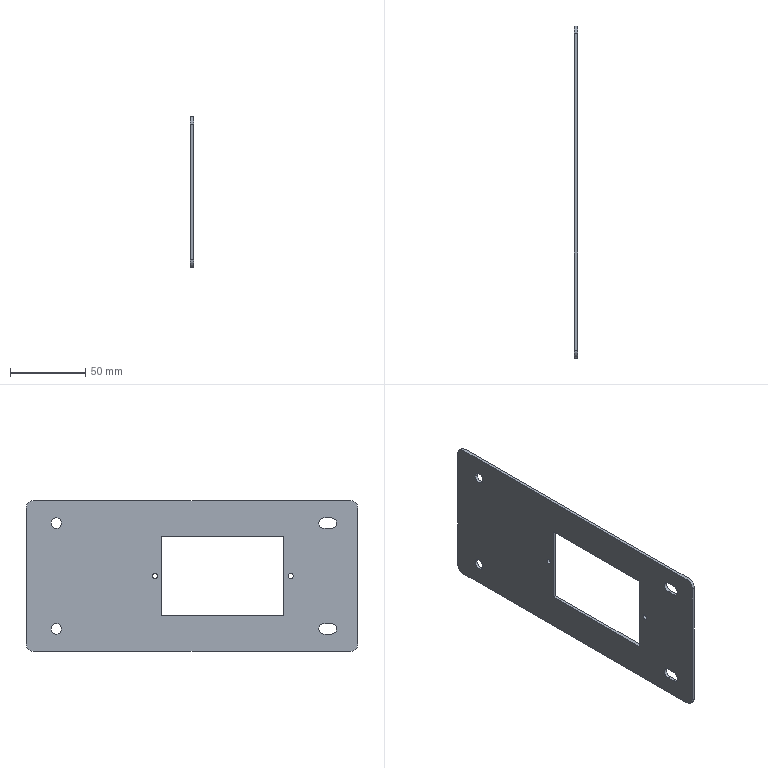Part | SolidWorks | features ExtruThin 1, Fillet 1, ICE 1 | 1 solid | 32 faces | box 2 x 220 x 100 mm | volume 34889 mm3 | cylinder 18 | plane 14 | commonest cylinder face diameters 7 x10 3.3 x4 10 x4
STEP:
#1=CARTESIAN_POINT('',(2.,14.,-85.));
#2=VERTEX_POINT('',#1);
#3=CARTESIAN_POINT('',(2.,17.5,-81.5));
#4=VERTEX_POINT('',#3);
#5=CARTESIAN_POINT('',(2.,17.5,-85.));
#6=DIRECTION('',(-1.,0.,0.));
#7=DIRECTION('',(0.,-1.,0.));
#8=AXIS2_PLACEMENT_3D('',#5,#6,#7);
#9=CIRCLE('',#8,3.5);
#10=EDGE_CURVE('',#2,#4,#9,.T.);
#11=ORIENTED_EDGE('',*,*,#10,.F.);
#12=CARTESIAN_POINT('',(0.,14.,-85.));
#13=VERTEX_POINT('',#12);
#14=CARTESIAN_POINT('',(10.,14.,-85.));
#15=DIRECTION('',(-1.,0.,0.));
#16=VECTOR('',#15,1000.);
#17=LINE('',#14,#16);
#18=EDGE_CURVE('',#2,#13,#17,.T.);
#19=ORIENTED_EDGE('',*,*,#18,.T.);
#20=CARTESIAN_POINT('',(0.,17.5,-81.5));
#21=VERTEX_POINT('',#20);
#22=CARTESIAN_POINT('',(0.,17.5,-85.));
#23=DIRECTION('',(-1.,0.,0.));
#24=DIRECTION('',(0.,-1.,0.));
#25=AXIS2_PLACEMENT_3D('',#22,#23,#24);
#26=CIRCLE('',#25,3.5);
#27=EDGE_CURVE('',#13,#21,#26,.T.);
#28=ORIENTED_EDGE('',*,*,#27,.T.);
#29=CARTESIAN_POINT('',(10.,17.5,-81.5));
#30=DIRECTION('',(-1.,0.,0.));
#31=VECTOR('',#30,1000.);
#32=LINE('',#29,#31);
#33=EDGE_CURVE('',#4,#21,#32,.T.);
#34=ORIENTED_EDGE('',*,*,#33,.F.);
#35=EDGE_LOOP('',(#11,#19,#28,#34));
#36=FACE_OUTER_BOUND('',#35,.T.);
#37=CARTESIAN_POINT('',(10.,17.5,-85.));
#38=DIRECTION('',(-1.,0.,0.));
#39=DIRECTION('',(0.,-1.,0.));
#40=AXIS2_PLACEMENT_3D('',#37,#38,#39);
#41=CYLINDRICAL_SURFACE('',#40,3.5);
#42=ADVANCED_FACE('',(#36),#41,.F.);
#43=CARTESIAN_POINT('',(2.,14.,-15.));
#44=VERTEX_POINT('',#43);
#45=CARTESIAN_POINT('',(2.,17.5,-11.5));
#46=VERTEX_POINT('',#45);
#47=CARTESIAN_POINT('',(2.,17.5,-15.));
#48=DIRECTION('',(-1.,0.,0.));
#49=DIRECTION('',(0.,-1.,0.));
#50=AXIS2_PLACEMENT_3D('',#47,#48,#49);
#51=CIRCLE('',#50,3.5);
#52=EDGE_CURVE('',#44,#46,#51,.T.);
#53=ORIENTED_EDGE('',*,*,#52,.F.);
#54=CARTESIAN_POINT('',(0.,14.,-15.));
#55=VERTEX_POINT('',#54);
#56=CARTESIAN_POINT('',(10.,14.,-15.));
#57=DIRECTION('',(-1.,0.,0.));
#58=VECTOR('',#57,1000.);
#59=LINE('',#56,#58);
#60=EDGE_CURVE('',#44,#55,#59,.T.);
#61=ORIENTED_EDGE('',*,*,#60,.T.);
#62=CARTESIAN_POINT('',(0.,17.5,-11.5));
#63=VERTEX_POINT('',#62);
#64=CARTESIAN_POINT('',(0.,17.5,-15.));
#65=DIRECTION('',(-1.,0.,0.));
#66=DIRECTION('',(0.,-1.,0.));
#67=AXIS2_PLACEMENT_3D('',#64,#65,#66);
#68=CIRCLE('',#67,3.5);
#69=EDGE_CURVE('',#55,#63,#68,.T.);
#70=ORIENTED_EDGE('',*,*,#69,.T.);
#71=CARTESIAN_POINT('',(10.,17.5,-11.5));
#72=DIRECTION('',(-1.,0.,0.));
#73=VECTOR('',#72,1000.);
#74=LINE('',#71,#73);
#75=EDGE_CURVE('',#46,#63,#74,.T.);
#76=ORIENTED_EDGE('',*,*,#75,.F.);
#77=EDGE_LOOP('',(#53,#61,#70,#76));
#78=FACE_OUTER_BOUND('',#77,.T.);
#79=CARTESIAN_POINT('',(10.,17.5,-15.));
#80=DIRECTION('',(-1.,0.,0.));
#81=DIRECTION('',(0.,-1.,0.));
#82=AXIS2_PLACEMENT_3D('',#79,#80,#81);
#83=CYLINDRICAL_SURFACE('',#82,3.5);
#84=ADVANCED_FACE('',(#78),#83,.F.);
#85=CARTESIAN_POINT('',(2.,203.5,-85.));
#86=VERTEX_POINT('',#85);
#87=CARTESIAN_POINT('',(2.,196.5,-85.));
#88=VERTEX_POINT('',#87);
#89=CARTESIAN_POINT('',(2.,200.,-85.));
#90=DIRECTION('',(-1.,0.,0.));
#91=DIRECTION('',(0.,-1.,0.));
#92=AXIS2_PLACEMENT_3D('',#89,#90,#91);
#93=CIRCLE('',#92,3.5);
#94=EDGE_CURVE('',#86,#88,#93,.T.);
#95=ORIENTED_EDGE('',*,*,#94,.F.);
#96=CARTESIAN_POINT('',(0.,203.5,-85.));
#97=VERTEX_POINT('',#96);
#98=CARTESIAN_POINT('',(10.,203.5,-85.));
#99=DIRECTION('',(-1.,0.,0.));
#100=VECTOR('',#99,1000.);
#101=LINE('',#98,#100);
#102=EDGE_CURVE('',#86,#97,#101,.T.);
#103=ORIENTED_EDGE('',*,*,#102,.T.);
#104=CARTESIAN_POINT('',(0.,196.5,-85.));
#105=VERTEX_POINT('',#104);
#106=CARTESIAN_POINT('',(0.,200.,-85.));
#107=DIRECTION('',(-1.,0.,0.));
#108=DIRECTION('',(0.,-1.,0.));
#109=AXIS2_PLACEMENT_3D('',#106,#107,#108);
#110=CIRCLE('',#109,3.5);
#111=EDGE_CURVE('',#97,#105,#110,.T.);
#112=ORIENTED_EDGE('',*,*,#111,.T.);
#113=CARTESIAN_POINT('',(10.,196.5,-85.));
#114=DIRECTION('',(-1.,0.,0.));
#115=VECTOR('',#114,1000.);
#116=LINE('',#113,#115);
#117=EDGE_CURVE('',#88,#105,#116,.T.);
#118=ORIENTED_EDGE('',*,*,#117,.F.);
#119=EDGE_LOOP('',(#95,#103,#112,#118));
#120=FACE_OUTER_BOUND('',#119,.T.);
#121=CARTESIAN_POINT('',(10.,200.,-85.));
#122=DIRECTION('',(-1.,0.,0.));
#123=DIRECTION('',(0.,-1.,0.));
#124=AXIS2_PLACEMENT_3D('',#121,#122,#123);
#125=CYLINDRICAL_SURFACE('',#124,3.5);
#126=ADVANCED_FACE('',(#120),#125,.F.);
#127=CARTESIAN_POINT('',(2.,203.5,-15.));
#128=VERTEX_POINT('',#127);
#129=CARTESIAN_POINT('',(2.,196.5,-15.));
#130=VERTEX_POINT('',#129);
#131=CARTESIAN_POINT('',(2.,200.,-15.));
#132=DIRECTION('',(-1.,0.,0.));
#133=DIRECTION('',(0.,-1.,0.));
#134=AXIS2_PLACEMENT_3D('',#131,#132,#133);
#135=CIRCLE('',#134,3.5);
#136=EDGE_CURVE('',#128,#130,#135,.T.);
#137=ORIENTED_EDGE('',*,*,#136,.F.);
#138=CARTESIAN_POINT('',(0.,203.5,-15.));
#139=VERTEX_POINT('',#138);
#140=CARTESIAN_POINT('',(10.,203.5,-15.));
#141=DIRECTION('',(-1.,0.,0.));
#142=VECTOR('',#141,1000.);
#143=LINE('',#140,#142);
#144=EDGE_CURVE('',#128,#139,#143,.T.);
#145=ORIENTED_EDGE('',*,*,#144,.T.);
#146=CARTESIAN_POINT('',(0.,196.5,-15.));
#147=VERTEX_POINT('',#146);
#148=CARTESIAN_POINT('',(0.,200.,-15.));
#149=DIRECTION('',(-1.,0.,0.));
#150=DIRECTION('',(0.,-1.,0.));
#151=AXIS2_PLACEMENT_3D('',#148,#149,#150);
#152=CIRCLE('',#151,3.5);
#153=EDGE_CURVE('',#139,#147,#152,.T.);
#154=ORIENTED_EDGE('',*,*,#153,.T.);
#155=CARTESIAN_POINT('',(10.,196.5,-15.));
#156=DIRECTION('',(-1.,0.,0.));
#157=VECTOR('',#156,1000.);
#158=LINE('',#155,#157);
#159=EDGE_CURVE('',#130,#147,#158,.T.);
#160=ORIENTED_EDGE('',*,*,#159,.F.);
#161=EDGE_LOOP('',(#137,#145,#154,#160));
#162=FACE_OUTER_BOUND('',#161,.T.);
#163=CARTESIAN_POINT('',(10.,200.,-15.));
#164=DIRECTION('',(-1.,0.,0.));
#165=DIRECTION('',(0.,-1.,0.));
#166=AXIS2_PLACEMENT_3D('',#163,#164,#165);
#167=CYLINDRICAL_SURFACE('',#166,3.5);
#168=ADVANCED_FACE('',(#162),#167,.F.);
#169=CARTESIAN_POINT('',(2.,136.15,-50.));
#170=VERTEX_POINT('',#169);
#171=CARTESIAN_POINT('',(2.,132.85,-50.));
#172=VERTEX_POINT('',#171);
#173=CARTESIAN_POINT('',(2.,134.5,-50.));
#174=DIRECTION('',(-1.,0.,0.));
#175=DIRECTION('',(0.,-1.,0.));
#176=AXIS2_PLACEMENT_3D('',#173,#174,#175);
#177=CIRCLE('',#176,1.65);
#178=EDGE_CURVE('',#170,#172,#177,.T.);
#179=ORIENTED_EDGE('',*,*,#178,.F.);
#180=CARTESIAN_POINT('',(0.,136.15,-50.));
#181=VERTEX_POINT('',#180);
#182=CARTESIAN_POINT('',(10.,136.15,-50.));
#183=DIRECTION('',(-1.,0.,0.));
#184=VECTOR('',#183,1000.);
#185=LINE('',#182,#184);
#186=EDGE_CURVE('',#170,#181,#185,.T.);
#187=ORIENTED_EDGE('',*,*,#186,.T.);
#188=CARTESIAN_POINT('',(0.,132.85,-50.));
#189=VERTEX_POINT('',#188);
#190=CARTESIAN_POINT('',(0.,134.5,-50.));
#191=DIRECTION('',(-1.,0.,0.));
#192=DIRECTION('',(0.,-1.,0.));
#193=AXIS2_PLACEMENT_3D('',#190,#191,#192);
#194=CIRCLE('',#193,1.65);
#195=EDGE_CURVE('',#181,#189,#194,.T.);
#196=ORIENTED_EDGE('',*,*,#195,.T.);
#197=CARTESIAN_POINT('',(10.,132.85,-50.));
#198=DIRECTION('',(-1.,0.,0.));
#199=VECTOR('',#198,1000.);
#200=LINE('',#197,#199);
#201=EDGE_CURVE('',#172,#189,#200,.T.);
#202=ORIENTED_EDGE('',*,*,#201,.F.);
#203=EDGE_LOOP('',(#179,#187,#196,#202));
#204=FACE_OUTER_BOUND('',#203,.T.);
#205=CARTESIAN_POINT('',(10.,134.5,-50.));
#206=DIRECTION('',(-1.,0.,0.));
#207=DIRECTION('',(0.,-1.,0.));
#208=AXIS2_PLACEMENT_3D('',#205,#206,#207);
#209=CYLINDRICAL_SURFACE('',#208,1.65);
#210=ADVANCED_FACE('',(#204),#209,.F.);
#211=CARTESIAN_POINT('',(2.,46.15,-50.));
#212=VERTEX_POINT('',#211);
#213=CARTESIAN_POINT('',(2.,42.85,-50.));
#214=VERTEX_POINT('',#213);
#215=CARTESIAN_POINT('',(2.,44.5,-50.));
#216=DIRECTION('',(-1.,0.,0.));
#217=DIRECTION('',(0.,-1.,0.));
#218=AXIS2_PLACEMENT_3D('',#215,#216,#217);
#219=CIRCLE('',#218,1.65);
#220=EDGE_CURVE('',#212,#214,#219,.T.);
#221=ORIENTED_EDGE('',*,*,#220,.F.);
#222=CARTESIAN_POINT('',(0.,46.15,-50.));
#223=VERTEX_POINT('',#222);
#224=CARTESIAN_POINT('',(10.,46.15,-50.));
#225=DIRECTION('',(-1.,0.,0.));
#226=VECTOR('',#225,1000.);
#227=LINE('',#224,#226);
#228=EDGE_CURVE('',#212,#223,#227,.T.);
#229=ORIENTED_EDGE('',*,*,#228,.T.);
#230=CARTESIAN_POINT('',(0.,42.85,-50.));
#231=VERTEX_POINT('',#230);
#232=CARTESIAN_POINT('',(0.,44.5,-50.));
#233=DIRECTION('',(-1.,0.,0.));
#234=DIRECTION('',(0.,-1.,0.));
#235=AXIS2_PLACEMENT_3D('',#232,#233,#234);
#236=CIRCLE('',#235,1.65);
#237=EDGE_CURVE('',#223,#231,#236,.T.);
#238=ORIENTED_EDGE('',*,*,#237,.T.);
#239=CARTESIAN_POINT('',(10.,42.85,-50.));
#240=DIRECTION('',(-1.,0.,0.));
#241=VECTOR('',#240,1000.);
#242=LINE('',#239,#241);
#243=EDGE_CURVE('',#214,#231,#242,.T.);
#244=ORIENTED_EDGE('',*,*,#243,.F.);
#245=EDGE_LOOP('',(#221,#229,#238,#244));
#246=FACE_OUTER_BOUND('',#245,.T.);
#247=CARTESIAN_POINT('',(10.,44.5,-50.));
#248=DIRECTION('',(-1.,0.,0.));
#249=DIRECTION('',(0.,-1.,0.));
#250=AXIS2_PLACEMENT_3D('',#247,#248,#249);
#251=CYLINDRICAL_SURFACE('',#250,1.65);
#252=ADVANCED_FACE('',(#246),#251,.F.);
#253=CARTESIAN_POINT('',(0.,22.5,-81.5));
#254=VERTEX_POINT('',#253);
#255=CARTESIAN_POINT('',(0.,22.5,-88.5));
#256=VERTEX_POINT('',#255);
#257=CARTESIAN_POINT('',(0.,22.5,-85.));
#258=DIRECTION('',(-1.,0.,0.));
#259=DIRECTION('',(0.,-1.,0.));
#260=AXIS2_PLACEMENT_3D('',#257,#258,#259);
#261=CIRCLE('',#260,3.5);
#262=EDGE_CURVE('',#254,#256,#261,.T.);
#263=ORIENTED_EDGE('',*,*,#262,.F.);
#264=CARTESIAN_POINT('',(0.,22.5,-81.5));
#265=DIRECTION('',(0.,1.,0.));
#266=VECTOR('',#265,1000.);
#267=LINE('',#264,#266);
#268=EDGE_CURVE('',#21,#254,#267,.T.);
#269=ORIENTED_EDGE('',*,*,#268,.F.);
#270=ORIENTED_EDGE('',*,*,#27,.F.);
#271=CARTESIAN_POINT('',(0.,17.5,-88.5));
#272=VERTEX_POINT('',#271);
#273=CARTESIAN_POINT('',(0.,17.5,-85.));
#274=DIRECTION('',(-1.,0.,0.));
#275=DIRECTION('',(0.,-1.,0.));
#276=AXIS2_PLACEMENT_3D('',#273,#274,#275);
#277=CIRCLE('',#276,3.5);
#278=EDGE_CURVE('',#272,#13,#277,.T.);
#279=ORIENTED_EDGE('',*,*,#278,.F.);
#280=CARTESIAN_POINT('',(0.,22.5,-88.5));
#281=DIRECTION('',(0.,-1.,0.));
#282=VECTOR('',#281,1000.);
#283=LINE('',#280,#282);
#284=EDGE_CURVE('',#256,#272,#283,.T.);
#285=ORIENTED_EDGE('',*,*,#284,.F.);
#286=EDGE_LOOP('',(#263,#269,#270,#279,#285));
#287=FACE_BOUND('',#286,.T.);
#288=CARTESIAN_POINT('',(0.,22.5,-11.5));
#289=VERTEX_POINT('',#288);
#290=CARTESIAN_POINT('',(0.,22.5,-18.5));
#291=VERTEX_POINT('',#290);
#292=CARTESIAN_POINT('',(0.,22.5,-15.));
#293=DIRECTION('',(-1.,0.,0.));
#294=DIRECTION('',(0.,-1.,0.));
#295=AXIS2_PLACEMENT_3D('',#292,#293,#294);
#296=CIRCLE('',#295,3.5);
#297=EDGE_CURVE('',#289,#291,#296,.T.);
#298=ORIENTED_EDGE('',*,*,#297,.F.);
#299=CARTESIAN_POINT('',(0.,22.5,-11.5));
#300=DIRECTION('',(0.,1.,0.));
#301=VECTOR('',#300,1000.);
#302=LINE('',#299,#301);
#303=EDGE_CURVE('',#63,#289,#302,.T.);
#304=ORIENTED_EDGE('',*,*,#303,.F.);
#305=ORIENTED_EDGE('',*,*,#69,.F.);
#306=CARTESIAN_POINT('',(0.,17.5,-18.5));
#307=VERTEX_POINT('',#306);
#308=CARTESIAN_POINT('',(0.,17.5,-15.));
#309=DIRECTION('',(-1.,0.,0.));
#310=DIRECTION('',(0.,-1.,0.));
#311=AXIS2_PLACEMENT_3D('',#308,#309,#310);
#312=CIRCLE('',#311,3.5);
#313=EDGE_CURVE('',#307,#55,#312,.T.);
#314=ORIENTED_EDGE('',*,*,#313,.F.);
#315=CARTESIAN_POINT('',(0.,22.5,-18.5));
#316=DIRECTION('',(0.,-1.,0.));
#317=VECTOR('',#316,1000.);
#318=LINE('',#315,#317);
#319=EDGE_CURVE('',#291,#307,#318,.T.);
#320=ORIENTED_EDGE('',*,*,#319,.F.);
#321=EDGE_LOOP('',(#298,#304,#305,#314,#320));
#322=FACE_BOUND('',#321,.T.);
#323=CARTESIAN_POINT('',(0.,200.,-85.));
#324=DIRECTION('',(-1.,0.,0.));
#325=DIRECTION('',(0.,-1.,0.));
#326=AXIS2_PLACEMENT_3D('',#323,#324,#325);
#327=CIRCLE('',#326,3.5);
#328=EDGE_CURVE('',#105,#97,#327,.T.);
#329=ORIENTED_EDGE('',*,*,#328,.F.);
#330=ORIENTED_EDGE('',*,*,#111,.F.);
#331=EDGE_LOOP('',(#329,#330));
#332=FACE_BOUND('',#331,.T.);
#333=CARTESIAN_POINT('',(0.,200.,-15.));
#334=DIRECTION('',(-1.,0.,0.));
#335=DIRECTION('',(0.,-1.,0.));
#336=AXIS2_PLACEMENT_3D('',#333,#334,#335);
#337=CIRCLE('',#336,3.5);
#338=EDGE_CURVE('',#147,#139,#337,.T.);
#339=ORIENTED_EDGE('',*,*,#338,.F.);
#340=ORIENTED_EDGE('',*,*,#153,.F.);
#341=EDGE_LOOP('',(#339,#340));
#342=FACE_BOUND('',#341,.T.);
#343=CARTESIAN_POINT('',(0.,134.5,-50.));
#344=DIRECTION('',(-1.,0.,0.));
#345=DIRECTION('',(0.,-1.,0.));
#346=AXIS2_PLACEMENT_3D('',#343,#344,#345);
#347=CIRCLE('',#346,1.65);
#348=EDGE_CURVE('',#189,#181,#347,.T.);
#349=ORIENTED_EDGE('',*,*,#348,.F.);
#350=ORIENTED_EDGE('',*,*,#195,.F.);
#351=EDGE_LOOP('',(#349,#350));
#352=FACE_BOUND('',#351,.T.);
#353=CARTESIAN_POINT('',(0.,44.5,-50.));
#354=DIRECTION('',(-1.,0.,0.));
#355=DIRECTION('',(0.,-1.,0.));
#356=AXIS2_PLACEMENT_3D('',#353,#354,#355);
#357=CIRCLE('',#356,1.65);
#358=EDGE_CURVE('',#231,#223,#357,.T.);
#359=ORIENTED_EDGE('',*,*,#358,.F.);
#360=ORIENTED_EDGE('',*,*,#237,.F.);
#361=EDGE_LOOP('',(#359,#360));
#362=FACE_BOUND('',#361,.T.);
#363=CARTESIAN_POINT('',(0.,130.,-76.5));
#364=VERTEX_POINT('',#363);
#365=CARTESIAN_POINT('',(0.,49.,-76.5));
#366=VERTEX_POINT('',#365);
#367=CARTESIAN_POINT('',(0.,130.,-76.5));
#368=DIRECTION('',(0.,-1.,0.));
#369=VECTOR('',#368,1000.);
#370=LINE('',#367,#369);
#371=EDGE_CURVE('',#364,#366,#370,.T.);
#372=ORIENTED_EDGE('',*,*,#371,.F.);
#373=CARTESIAN_POINT('',(0.,130.,-23.5));
#374=VERTEX_POINT('',#373);
#375=CARTESIAN_POINT('',(0.,130.,-23.5));
#376=DIRECTION('',(0.,0.,-1.));
#377=VECTOR('',#376,1000.);
#378=LINE('',#375,#377);
#379=EDGE_CURVE('',#374,#364,#378,.T.);
#380=ORIENTED_EDGE('',*,*,#379,.F.);
#381=CARTESIAN_POINT('',(0.,49.,-23.5));
#382=VERTEX_POINT('',#381);
#383=CARTESIAN_POINT('',(0.,130.,-23.5));
#384=DIRECTION('',(0.,1.,0.));
#385=VECTOR('',#384,1000.);
#386=LINE('',#383,#385);
#387=EDGE_CURVE('',#382,#374,#386,.T.);
#388=ORIENTED_EDGE('',*,*,#387,.F.);
#389=CARTESIAN_POINT('',(0.,49.,-23.5));
#390=DIRECTION('',(0.,0.,1.));
#391=VECTOR('',#390,1000.);
#392=LINE('',#389,#391);
#393=EDGE_CURVE('',#366,#382,#392,.T.);
#394=ORIENTED_EDGE('',*,*,#393,.F.);
#395=EDGE_LOOP('',(#372,#380,#388,#394));
#396=FACE_BOUND('',#395,.T.);
#397=CARTESIAN_POINT('',(0.,220.,-95.));
#398=VERTEX_POINT('',#397);
#399=CARTESIAN_POINT('',(0.,220.,-5.));
#400=VERTEX_POINT('',#399);
#401=CARTESIAN_POINT('',(0.,220.,-100.));
#402=DIRECTION('',(0.,0.,1.));
#403=VECTOR('',#402,1000.);
#404=LINE('',#401,#403);
#405=EDGE_CURVE('',#398,#400,#404,.T.);
#406=ORIENTED_EDGE('',*,*,#405,.F.);
#407=CARTESIAN_POINT('',(0.,215.,-100.));
#408=VERTEX_POINT('',#407);
#409=CARTESIAN_POINT('',(0.,215.,-95.));
#410=DIRECTION('',(-1.,0.,0.));
#411=DIRECTION('',(0.,-1.,0.));
#412=AXIS2_PLACEMENT_3D('',#409,#410,#411);
#413=CIRCLE('',#412,5.);
#414=EDGE_CURVE('',#398,#408,#413,.T.);
#415=ORIENTED_EDGE('',*,*,#414,.T.);
#416=CARTESIAN_POINT('',(0.,5.,-100.));
#417=VERTEX_POINT('',#416);
#418=CARTESIAN_POINT('',(0.,220.,-100.));
#419=DIRECTION('',(0.,-1.,0.));
#420=VECTOR('',#419,1000.);
#421=LINE('',#418,#420);
#422=EDGE_CURVE('',#408,#417,#421,.T.);
#423=ORIENTED_EDGE('',*,*,#422,.T.);
#424=CARTESIAN_POINT('',(0.,0.,-95.));
#425=VERTEX_POINT('',#424);
#426=CARTESIAN_POINT('',(0.,5.,-95.));
#427=DIRECTION('',(-1.,0.,0.));
#428=DIRECTION('',(0.,-1.,0.));
#429=AXIS2_PLACEMENT_3D('',#426,#427,#428);
#430=CIRCLE('',#429,5.);
#431=EDGE_CURVE('',#417,#425,#430,.T.);
#432=ORIENTED_EDGE('',*,*,#431,.T.);
#433=CARTESIAN_POINT('',(0.,0.,-5.));
#434=VERTEX_POINT('',#433);
#435=CARTESIAN_POINT('',(0.,0.,-100.));
#436=DIRECTION('',(0.,0.,1.));
#437=VECTOR('',#436,1000.);
#438=LINE('',#435,#437);
#439=EDGE_CURVE('',#425,#434,#438,.T.);
#440=ORIENTED_EDGE('',*,*,#439,.T.);
#441=CARTESIAN_POINT('',(0.,5.,0.));
#442=VERTEX_POINT('',#441);
#443=CARTESIAN_POINT('',(0.,5.,-5.));
#444=DIRECTION('',(-1.,0.,0.));
#445=DIRECTION('',(0.,-1.,0.));
#446=AXIS2_PLACEMENT_3D('',#443,#444,#445);
#447=CIRCLE('',#446,5.);
#448=EDGE_CURVE('',#434,#442,#447,.T.);
#449=ORIENTED_EDGE('',*,*,#448,.T.);
#450=CARTESIAN_POINT('',(0.,215.,0.));
#451=VERTEX_POINT('',#450);
#452=CARTESIAN_POINT('',(0.,220.,0.));
#453=DIRECTION('',(0.,-1.,0.));
#454=VECTOR('',#453,1000.);
#455=LINE('',#452,#454);
#456=EDGE_CURVE('',#451,#442,#455,.T.);
#457=ORIENTED_EDGE('',*,*,#456,.F.);
#458=CARTESIAN_POINT('',(0.,215.,-5.));
#459=DIRECTION('',(-1.,0.,0.));
#460=DIRECTION('',(0.,-1.,0.));
#461=AXIS2_PLACEMENT_3D('',#458,#459,#460);
#462=CIRCLE('',#461,5.);
#463=EDGE_CURVE('',#451,#400,#462,.T.);
#464=ORIENTED_EDGE('',*,*,#463,.T.);
#465=EDGE_LOOP('',(#406,#415,#423,#432,#440,#449,#457,#464));
#466=FACE_OUTER_BOUND('',#465,.T.);
#467=CARTESIAN_POINT('',(0.,220.,-100.));
#468=DIRECTION('',(-1.,0.,0.));
#469=DIRECTION('',(0.,-1.,0.));
#470=AXIS2_PLACEMENT_3D('',#467,#468,#469);
#471=PLANE('',#470);
#472=ADVANCED_FACE('',(#287,#322,#332,#342,#352,#362,#396,#466),#471,.T.);
#473=CARTESIAN_POINT('',(2.,220.,-95.));
#474=VERTEX_POINT('',#473);
#475=CARTESIAN_POINT('',(2.,220.,-5.));
#476=VERTEX_POINT('',#475);
#477=CARTESIAN_POINT('',(2.,220.,-100.));
#478=DIRECTION('',(0.,0.,1.));
#479=VECTOR('',#478,1000.);
#480=LINE('',#477,#479);
#481=EDGE_CURVE('',#474,#476,#480,.T.);
#482=ORIENTED_EDGE('',*,*,#481,.F.);
#483=CARTESIAN_POINT('',(0.,220.,-95.));
#484=DIRECTION('',(-1.,0.,0.));
#485=VECTOR('',#484,1000.);
#486=LINE('',#483,#485);
#487=EDGE_CURVE('',#474,#398,#486,.T.);
#488=ORIENTED_EDGE('',*,*,#487,.T.);
#489=ORIENTED_EDGE('',*,*,#405,.T.);
#490=CARTESIAN_POINT('',(0.,220.,-5.));
#491=DIRECTION('',(1.,0.,0.));
#492=VECTOR('',#491,1000.);
#493=LINE('',#490,#492);
#494=EDGE_CURVE('',#400,#476,#493,.T.);
#495=ORIENTED_EDGE('',*,*,#494,.T.);
#496=EDGE_LOOP('',(#482,#488,#489,#495));
#497=FACE_OUTER_BOUND('',#496,.T.);
#498=CARTESIAN_POINT('',(0.,220.,-100.));
#499=DIRECTION('',(0.,-1.,0.));
#500=DIRECTION('',(0.,0.,-1.));
#501=AXIS2_PLACEMENT_3D('',#498,#499,#500);
#502=PLANE('',#501);
#503=ADVANCED_FACE('',(#497),#502,.F.);
#504=CARTESIAN_POINT('',(2.,22.5,-81.5));
#505=VERTEX_POINT('',#504);
#506=CARTESIAN_POINT('',(2.,220.,-81.5));
#507=DIRECTION('',(0.,1.,0.));
#508=VECTOR('',#507,1000.);
#509=LINE('',#506,#508);
#510=EDGE_CURVE('',#4,#505,#509,.T.);
#511=ORIENTED_EDGE('',*,*,#510,.T.);
#512=CARTESIAN_POINT('',(2.,22.5,-88.5));
#513=VERTEX_POINT('',#512);
#514=CARTESIAN_POINT('',(2.,22.5,-85.));
#515=DIRECTION('',(-1.,0.,0.));
#516=DIRECTION('',(0.,-1.,0.));
#517=AXIS2_PLACEMENT_3D('',#514,#515,#516);
#518=CIRCLE('',#517,3.5);
#519=EDGE_CURVE('',#505,#513,#518,.T.);
#520=ORIENTED_EDGE('',*,*,#519,.T.);
#521=CARTESIAN_POINT('',(2.,17.5,-88.5));
#522=VERTEX_POINT('',#521);
#523=CARTESIAN_POINT('',(2.,220.,-88.5));
#524=DIRECTION('',(0.,-1.,0.));
#525=VECTOR('',#524,1000.);
#526=LINE('',#523,#525);
#527=EDGE_CURVE('',#513,#522,#526,.T.);
#528=ORIENTED_EDGE('',*,*,#527,.T.);
#529=CARTESIAN_POINT('',(2.,17.5,-85.));
#530=DIRECTION('',(-1.,0.,0.));
#531=DIRECTION('',(0.,-1.,0.));
#532=AXIS2_PLACEMENT_3D('',#529,#530,#531);
#533=CIRCLE('',#532,3.5);
#534=EDGE_CURVE('',#522,#2,#533,.T.);
#535=ORIENTED_EDGE('',*,*,#534,.T.);
#536=ORIENTED_EDGE('',*,*,#10,.T.);
#537=EDGE_LOOP('',(#511,#520,#528,#535,#536));
#538=FACE_BOUND('',#537,.T.);
#539=CARTESIAN_POINT('',(2.,22.5,-11.5));
#540=VERTEX_POINT('',#539);
#541=CARTESIAN_POINT('',(2.,220.,-11.5));
#542=DIRECTION('',(0.,1.,0.));
#543=VECTOR('',#542,1000.);
#544=LINE('',#541,#543);
#545=EDGE_CURVE('',#46,#540,#544,.T.);
#546=ORIENTED_EDGE('',*,*,#545,.T.);
#547=CARTESIAN_POINT('',(2.,22.5,-18.5));
#548=VERTEX_POINT('',#547);
#549=CARTESIAN_POINT('',(2.,22.5,-15.));
#550=DIRECTION('',(-1.,0.,0.));
#551=DIRECTION('',(0.,-1.,0.));
#552=AXIS2_PLACEMENT_3D('',#549,#550,#551);
#553=CIRCLE('',#552,3.5);
#554=EDGE_CURVE('',#540,#548,#553,.T.);
#555=ORIENTED_EDGE('',*,*,#554,.T.);
#556=CARTESIAN_POINT('',(2.,17.5,-18.5));
#557=VERTEX_POINT('',#556);
#558=CARTESIAN_POINT('',(2.,220.,-18.5));
#559=DIRECTION('',(0.,-1.,0.));
#560=VECTOR('',#559,1000.);
#561=LINE('',#558,#560);
#562=EDGE_CURVE('',#548,#557,#561,.T.);
#563=ORIENTED_EDGE('',*,*,#562,.T.);
#564=CARTESIAN_POINT('',(2.,17.5,-15.));
#565=DIRECTION('',(-1.,0.,0.));
#566=DIRECTION('',(0.,-1.,0.));
#567=AXIS2_PLACEMENT_3D('',#564,#565,#566);
#568=CIRCLE('',#567,3.5);
#569=EDGE_CURVE('',#557,#44,#568,.T.);
#570=ORIENTED_EDGE('',*,*,#569,.T.);
#571=ORIENTED_EDGE('',*,*,#52,.T.);
#572=EDGE_LOOP('',(#546,#555,#563,#570,#571));
#573=FACE_BOUND('',#572,.T.);
#574=CARTESIAN_POINT('',(2.,200.,-85.));
#575=DIRECTION('',(-1.,0.,0.));
#576=DIRECTION('',(0.,-1.,0.));
#577=AXIS2_PLACEMENT_3D('',#574,#575,#576);
#578=CIRCLE('',#577,3.5);
#579=EDGE_CURVE('',#88,#86,#578,.T.);
#580=ORIENTED_EDGE('',*,*,#579,.T.);
#581=ORIENTED_EDGE('',*,*,#94,.T.);
#582=EDGE_LOOP('',(#580,#581));
#583=FACE_BOUND('',#582,.T.);
#584=CARTESIAN_POINT('',(2.,200.,-15.));
#585=DIRECTION('',(-1.,0.,0.));
#586=DIRECTION('',(0.,-1.,0.));
#587=AXIS2_PLACEMENT_3D('',#584,#585,#586);
#588=CIRCLE('',#587,3.5);
#589=EDGE_CURVE('',#130,#128,#588,.T.);
#590=ORIENTED_EDGE('',*,*,#589,.T.);
#591=ORIENTED_EDGE('',*,*,#136,.T.);
#592=EDGE_LOOP('',(#590,#591));
#593=FACE_BOUND('',#592,.T.);
#594=CARTESIAN_POINT('',(2.,134.5,-50.));
#595=DIRECTION('',(-1.,0.,0.));
#596=DIRECTION('',(0.,-1.,0.));
#597=AXIS2_PLACEMENT_3D('',#594,#595,#596);
#598=CIRCLE('',#597,1.65);
#599=EDGE_CURVE('',#172,#170,#598,.T.);
#600=ORIENTED_EDGE('',*,*,#599,.T.);
#601=ORIENTED_EDGE('',*,*,#178,.T.);
#602=EDGE_LOOP('',(#600,#601));
#603=FACE_BOUND('',#602,.T.);
#604=CARTESIAN_POINT('',(2.,44.5,-50.));
#605=DIRECTION('',(-1.,0.,0.));
#606=DIRECTION('',(0.,-1.,0.));
#607=AXIS2_PLACEMENT_3D('',#604,#605,#606);
#608=CIRCLE('',#607,1.65);
#609=EDGE_CURVE('',#214,#212,#608,.T.);
#610=ORIENTED_EDGE('',*,*,#609,.T.);
#611=ORIENTED_EDGE('',*,*,#220,.T.);
#612=EDGE_LOOP('',(#610,#611));
#613=FACE_BOUND('',#612,.T.);
#614=CARTESIAN_POINT('',(2.,130.,-23.5));
#615=VERTEX_POINT('',#614);
#616=CARTESIAN_POINT('',(2.,130.,-76.5));
#617=VERTEX_POINT('',#616);
#618=CARTESIAN_POINT('',(2.,130.,-100.));
#619=DIRECTION('',(0.,0.,-1.));
#620=VECTOR('',#619,1000.);
#621=LINE('',#618,#620);
#622=EDGE_CURVE('',#615,#617,#621,.T.);
#623=ORIENTED_EDGE('',*,*,#622,.T.);
#624=CARTESIAN_POINT('',(2.,49.,-76.5));
#625=VERTEX_POINT('',#624);
#626=CARTESIAN_POINT('',(2.,220.,-76.5));
#627=DIRECTION('',(0.,-1.,0.));
#628=VECTOR('',#627,1000.);
#629=LINE('',#626,#628);
#630=EDGE_CURVE('',#617,#625,#629,.T.);
#631=ORIENTED_EDGE('',*,*,#630,.T.);
#632=CARTESIAN_POINT('',(2.,49.,-23.5));
#633=VERTEX_POINT('',#632);
#634=CARTESIAN_POINT('',(2.,49.,-100.));
#635=DIRECTION('',(0.,0.,1.));
#636=VECTOR('',#635,1000.);
#637=LINE('',#634,#636);
#638=EDGE_CURVE('',#625,#633,#637,.T.);
#639=ORIENTED_EDGE('',*,*,#638,.T.);
#640=CARTESIAN_POINT('',(2.,220.,-23.5));
#641=DIRECTION('',(0.,1.,0.));
#642=VECTOR('',#641,1000.);
#643=LINE('',#640,#642);
#644=EDGE_CURVE('',#633,#615,#643,.T.);
#645=ORIENTED_EDGE('',*,*,#644,.T.);
#646=EDGE_LOOP('',(#623,#631,#639,#645));
#647=FACE_BOUND('',#646,.T.);
#648=CARTESIAN_POINT('',(2.,215.,-100.));
#649=VERTEX_POINT('',#648);
#650=CARTESIAN_POINT('',(2.,5.,-100.));
#651=VERTEX_POINT('',#650);
#652=CARTESIAN_POINT('',(2.,220.,-100.));
#653=DIRECTION('',(0.,-1.,0.));
#654=VECTOR('',#653,1000.);
#655=LINE('',#652,#654);
#656=EDGE_CURVE('',#649,#651,#655,.T.);
#657=ORIENTED_EDGE('',*,*,#656,.F.);
#658=CARTESIAN_POINT('',(2.,215.,-95.));
#659=DIRECTION('',(1.,0.,0.));
#660=DIRECTION('',(0.,-1.,0.));
#661=AXIS2_PLACEMENT_3D('',#658,#659,#660);
#662=CIRCLE('',#661,5.);
#663=EDGE_CURVE('',#649,#474,#662,.T.);
#664=ORIENTED_EDGE('',*,*,#663,.T.);
#665=ORIENTED_EDGE('',*,*,#481,.T.);
#666=CARTESIAN_POINT('',(2.,215.,0.));
#667=VERTEX_POINT('',#666);
#668=CARTESIAN_POINT('',(2.,215.,-5.));
#669=DIRECTION('',(1.,0.,0.));
#670=DIRECTION('',(0.,-1.,0.));
#671=AXIS2_PLACEMENT_3D('',#668,#669,#670);
#672=CIRCLE('',#671,5.);
#673=EDGE_CURVE('',#476,#667,#672,.T.);
#674=ORIENTED_EDGE('',*,*,#673,.T.);
#675=CARTESIAN_POINT('',(2.,5.,0.));
#676=VERTEX_POINT('',#675);
#677=CARTESIAN_POINT('',(2.,220.,0.));
#678=DIRECTION('',(0.,-1.,0.));
#679=VECTOR('',#678,1000.);
#680=LINE('',#677,#679);
#681=EDGE_CURVE('',#667,#676,#680,.T.);
#682=ORIENTED_EDGE('',*,*,#681,.T.);
#683=CARTESIAN_POINT('',(2.,0.,-5.));
#684=VERTEX_POINT('',#683);
#685=CARTESIAN_POINT('',(2.,5.,-5.));
#686=DIRECTION('',(1.,0.,0.));
#687=DIRECTION('',(0.,-1.,0.));
#688=AXIS2_PLACEMENT_3D('',#685,#686,#687);
#689=CIRCLE('',#688,5.);
#690=EDGE_CURVE('',#676,#684,#689,.T.);
#691=ORIENTED_EDGE('',*,*,#690,.T.);
#692=CARTESIAN_POINT('',(2.,0.,-95.));
#693=VERTEX_POINT('',#692);
#694=CARTESIAN_POINT('',(2.,0.,-100.));
#695=DIRECTION('',(0.,0.,1.));
#696=VECTOR('',#695,1000.);
#697=LINE('',#694,#696);
#698=EDGE_CURVE('',#693,#684,#697,.T.);
#699=ORIENTED_EDGE('',*,*,#698,.F.);
#700=CARTESIAN_POINT('',(2.,5.,-95.));
#701=DIRECTION('',(1.,0.,0.));
#702=DIRECTION('',(0.,-1.,0.));
#703=AXIS2_PLACEMENT_3D('',#700,#701,#702);
#704=CIRCLE('',#703,5.);
#705=EDGE_CURVE('',#693,#651,#704,.T.);
#706=ORIENTED_EDGE('',*,*,#705,.T.);
#707=EDGE_LOOP('',(#657,#664,#665,#674,#682,#691,#699,#706));
#708=FACE_OUTER_BOUND('',#707,.T.);
#709=CARTESIAN_POINT('',(2.,220.,-100.));
#710=DIRECTION('',(-1.,0.,0.));
#711=DIRECTION('',(0.,-1.,0.));
#712=AXIS2_PLACEMENT_3D('',#709,#710,#711);
#713=PLANE('',#712);
#714=ADVANCED_FACE('',(#538,#573,#583,#593,#603,#613,#647,#708),#713,.F.);
#715=ORIENTED_EDGE('',*,*,#439,.F.);
#716=CARTESIAN_POINT('',(2.,0.,-95.));
#717=DIRECTION('',(1.,0.,0.));
#718=VECTOR('',#717,1000.);
#719=LINE('',#716,#718);
#720=EDGE_CURVE('',#425,#693,#719,.T.);
#721=ORIENTED_EDGE('',*,*,#720,.T.);
#722=ORIENTED_EDGE('',*,*,#698,.T.);
#723=CARTESIAN_POINT('',(2.,0.,-5.));
#724=DIRECTION('',(-1.,0.,0.));
#725=VECTOR('',#724,1000.);
#726=LINE('',#723,#725);
#727=EDGE_CURVE('',#684,#434,#726,.T.);
#728=ORIENTED_EDGE('',*,*,#727,.T.);
#729=EDGE_LOOP('',(#715,#721,#722,#728));
#730=FACE_OUTER_BOUND('',#729,.T.);
#731=CARTESIAN_POINT('',(2.,0.,-100.));
#732=DIRECTION('',(0.,1.,0.));
#733=DIRECTION('',(0.,0.,1.));
#734=AXIS2_PLACEMENT_3D('',#731,#732,#733);
#735=PLANE('',#734);
#736=ADVANCED_FACE('',(#730),#735,.F.);
#737=ORIENTED_EDGE('',*,*,#422,.F.);
#738=CARTESIAN_POINT('',(2.,215.,-100.));
#739=DIRECTION('',(1.,0.,0.));
#740=VECTOR('',#739,1000.);
#741=LINE('',#738,#740);
#742=EDGE_CURVE('',#408,#649,#741,.T.);
#743=ORIENTED_EDGE('',*,*,#742,.T.);
#744=ORIENTED_EDGE('',*,*,#656,.T.);
#745=CARTESIAN_POINT('',(0.,5.,-100.));
#746=DIRECTION('',(-1.,0.,0.));
#747=VECTOR('',#746,1000.);
#748=LINE('',#745,#747);
#749=EDGE_CURVE('',#651,#417,#748,.T.);
#750=ORIENTED_EDGE('',*,*,#749,.T.);
#751=EDGE_LOOP('',(#737,#743,#744,#750));
#752=FACE_OUTER_BOUND('',#751,.T.);
#753=CARTESIAN_POINT('',(0.,0.,-100.));
#754=DIRECTION('',(0.,0.,-1.));
#755=DIRECTION('',(-1.,0.,0.));
#756=AXIS2_PLACEMENT_3D('',#753,#754,#755);
#757=PLANE('',#756);
#758=ADVANCED_FACE('',(#752),#757,.T.);
#759=ORIENTED_EDGE('',*,*,#456,.T.);
#760=CARTESIAN_POINT('',(0.,5.,0.));
#761=DIRECTION('',(1.,0.,0.));
#762=VECTOR('',#761,1000.);
#763=LINE('',#760,#762);
#764=EDGE_CURVE('',#442,#676,#763,.T.);
#765=ORIENTED_EDGE('',*,*,#764,.T.);
#766=ORIENTED_EDGE('',*,*,#681,.F.);
#767=CARTESIAN_POINT('',(0.,215.,0.));
#768=DIRECTION('',(-1.,0.,0.));
#769=VECTOR('',#768,1000.);
#770=LINE('',#767,#769);
#771=EDGE_CURVE('',#667,#451,#770,.T.);
#772=ORIENTED_EDGE('',*,*,#771,.T.);
#773=EDGE_LOOP('',(#759,#765,#766,#772));
#774=FACE_OUTER_BOUND('',#773,.T.);
#775=CARTESIAN_POINT('',(0.,0.,0.));
#776=DIRECTION('',(0.,0.,-1.));
#777=DIRECTION('',(-1.,0.,0.));
#778=AXIS2_PLACEMENT_3D('',#775,#776,#777);
#779=PLANE('',#778);
#780=ADVANCED_FACE('',(#774),#779,.F.);
#781=CARTESIAN_POINT('',(10.,130.,-76.5));
#782=DIRECTION('',(-1.,0.,0.));
#783=VECTOR('',#782,1000.);
#784=LINE('',#781,#783);
#785=EDGE_CURVE('',#617,#364,#784,.T.);
#786=ORIENTED_EDGE('',*,*,#785,.T.);
#787=ORIENTED_EDGE('',*,*,#371,.T.);
#788=CARTESIAN_POINT('',(10.,49.,-76.5));
#789=DIRECTION('',(-1.,0.,0.));
#790=VECTOR('',#789,1000.);
#791=LINE('',#788,#790);
#792=EDGE_CURVE('',#625,#366,#791,.T.);
#793=ORIENTED_EDGE('',*,*,#792,.F.);
#794=ORIENTED_EDGE('',*,*,#630,.F.);
#795=EDGE_LOOP('',(#786,#787,#793,#794));
#796=FACE_OUTER_BOUND('',#795,.T.);
#797=CARTESIAN_POINT('',(10.,130.,-76.5));
#798=DIRECTION('',(0.,0.,-1.));
#799=DIRECTION('',(0.,1.,0.));
#800=AXIS2_PLACEMENT_3D('',#797,#798,#799);
#801=PLANE('',#800);
#802=ADVANCED_FACE('',(#796),#801,.F.);
#803=CARTESIAN_POINT('',(10.,130.,-23.5));
#804=DIRECTION('',(-1.,0.,0.));
#805=VECTOR('',#804,1000.);
#806=LINE('',#803,#805);
#807=EDGE_CURVE('',#615,#374,#806,.T.);
#808=ORIENTED_EDGE('',*,*,#807,.T.);
#809=ORIENTED_EDGE('',*,*,#379,.T.);
#810=ORIENTED_EDGE('',*,*,#785,.F.);
#811=ORIENTED_EDGE('',*,*,#622,.F.);
#812=EDGE_LOOP('',(#808,#809,#810,#811));
#813=FACE_OUTER_BOUND('',#812,.T.);
#814=CARTESIAN_POINT('',(10.,130.,-23.5));
#815=DIRECTION('',(0.,1.,0.));
#816=DIRECTION('',(-1.,0.,0.));
#817=AXIS2_PLACEMENT_3D('',#814,#815,#816);
#818=PLANE('',#817);
#819=ADVANCED_FACE('',(#813),#818,.F.);
#820=CARTESIAN_POINT('',(10.,49.,-23.5));
#821=DIRECTION('',(-1.,0.,0.));
#822=VECTOR('',#821,1000.);
#823=LINE('',#820,#822);
#824=EDGE_CURVE('',#633,#382,#823,.T.);
#825=ORIENTED_EDGE('',*,*,#824,.T.);
#826=ORIENTED_EDGE('',*,*,#387,.T.);
#827=ORIENTED_EDGE('',*,*,#807,.F.);
#828=ORIENTED_EDGE('',*,*,#644,.F.);
#829=EDGE_LOOP('',(#825,#826,#827,#828));
#830=FACE_OUTER_BOUND('',#829,.T.);
#831=CARTESIAN_POINT('',(10.,130.,-23.5));
#832=DIRECTION('',(0.,0.,1.));
#833=DIRECTION('',(0.,-1.,0.));
#834=AXIS2_PLACEMENT_3D('',#831,#832,#833);
#835=PLANE('',#834);
#836=ADVANCED_FACE('',(#830),#835,.F.);
#837=ORIENTED_EDGE('',*,*,#792,.T.);
#838=ORIENTED_EDGE('',*,*,#393,.T.);
#839=ORIENTED_EDGE('',*,*,#824,.F.);
#840=ORIENTED_EDGE('',*,*,#638,.F.);
#841=EDGE_LOOP('',(#837,#838,#839,#840));
#842=FACE_OUTER_BOUND('',#841,.T.);
#843=CARTESIAN_POINT('',(10.,49.,-23.5));
#844=DIRECTION('',(0.,-1.,0.));
#845=DIRECTION('',(0.,0.,-1.));
#846=AXIS2_PLACEMENT_3D('',#843,#844,#845);
#847=PLANE('',#846);
#848=ADVANCED_FACE('',(#842),#847,.F.);
#849=ORIENTED_EDGE('',*,*,#228,.F.);
#850=ORIENTED_EDGE('',*,*,#609,.F.);
#851=ORIENTED_EDGE('',*,*,#243,.T.);
#852=ORIENTED_EDGE('',*,*,#358,.T.);
#853=EDGE_LOOP('',(#849,#850,#851,#852));
#854=FACE_OUTER_BOUND('',#853,.T.);
#855=CARTESIAN_POINT('',(10.,44.5,-50.));
#856=DIRECTION('',(-1.,0.,0.));
#857=DIRECTION('',(0.,-1.,0.));
#858=AXIS2_PLACEMENT_3D('',#855,#856,#857);
#859=CYLINDRICAL_SURFACE('',#858,1.65);
#860=ADVANCED_FACE('',(#854),#859,.F.);
#861=ORIENTED_EDGE('',*,*,#186,.F.);
#862=ORIENTED_EDGE('',*,*,#599,.F.);
#863=ORIENTED_EDGE('',*,*,#201,.T.);
#864=ORIENTED_EDGE('',*,*,#348,.T.);
#865=EDGE_LOOP('',(#861,#862,#863,#864));
#866=FACE_OUTER_BOUND('',#865,.T.);
#867=CARTESIAN_POINT('',(10.,134.5,-50.));
#868=DIRECTION('',(-1.,0.,0.));
#869=DIRECTION('',(0.,-1.,0.));
#870=AXIS2_PLACEMENT_3D('',#867,#868,#869);
#871=CYLINDRICAL_SURFACE('',#870,1.65);
#872=ADVANCED_FACE('',(#866),#871,.F.);
#873=ORIENTED_EDGE('',*,*,#144,.F.);
#874=ORIENTED_EDGE('',*,*,#589,.F.);
#875=ORIENTED_EDGE('',*,*,#159,.T.);
#876=ORIENTED_EDGE('',*,*,#338,.T.);
#877=EDGE_LOOP('',(#873,#874,#875,#876));
#878=FACE_OUTER_BOUND('',#877,.T.);
#879=CARTESIAN_POINT('',(10.,200.,-15.));
#880=DIRECTION('',(-1.,0.,0.));
#881=DIRECTION('',(0.,-1.,0.));
#882=AXIS2_PLACEMENT_3D('',#879,#880,#881);
#883=CYLINDRICAL_SURFACE('',#882,3.5);
#884=ADVANCED_FACE('',(#878),#883,.F.);
#885=ORIENTED_EDGE('',*,*,#102,.F.);
#886=ORIENTED_EDGE('',*,*,#579,.F.);
#887=ORIENTED_EDGE('',*,*,#117,.T.);
#888=ORIENTED_EDGE('',*,*,#328,.T.);
#889=EDGE_LOOP('',(#885,#886,#887,#888));
#890=FACE_OUTER_BOUND('',#889,.T.);
#891=CARTESIAN_POINT('',(10.,200.,-85.));
#892=DIRECTION('',(-1.,0.,0.));
#893=DIRECTION('',(0.,-1.,0.));
#894=AXIS2_PLACEMENT_3D('',#891,#892,#893);
#895=CYLINDRICAL_SURFACE('',#894,3.5);
#896=ADVANCED_FACE('',(#890),#895,.F.);
#897=CARTESIAN_POINT('',(10.,22.5,-11.5));
#898=DIRECTION('',(-1.,0.,0.));
#899=VECTOR('',#898,1000.);
#900=LINE('',#897,#899);
#901=EDGE_CURVE('',#540,#289,#900,.T.);
#902=ORIENTED_EDGE('',*,*,#901,.T.);
#903=ORIENTED_EDGE('',*,*,#297,.T.);
#904=CARTESIAN_POINT('',(10.,22.5,-18.5));
#905=DIRECTION('',(-1.,0.,0.));
#906=VECTOR('',#905,1000.);
#907=LINE('',#904,#906);
#908=EDGE_CURVE('',#548,#291,#907,.T.);
#909=ORIENTED_EDGE('',*,*,#908,.F.);
#910=ORIENTED_EDGE('',*,*,#554,.F.);
#911=EDGE_LOOP('',(#902,#903,#909,#910));
#912=FACE_OUTER_BOUND('',#911,.T.);
#913=CARTESIAN_POINT('',(10.,22.5,-15.));
#914=DIRECTION('',(-1.,0.,0.));
#915=DIRECTION('',(0.,-1.,0.));
#916=AXIS2_PLACEMENT_3D('',#913,#914,#915);
#917=CYLINDRICAL_SURFACE('',#916,3.5);
#918=ADVANCED_FACE('',(#912),#917,.F.);
#919=ORIENTED_EDGE('',*,*,#75,.T.);
#920=ORIENTED_EDGE('',*,*,#303,.T.);
#921=ORIENTED_EDGE('',*,*,#901,.F.);
#922=ORIENTED_EDGE('',*,*,#545,.F.);
#923=EDGE_LOOP('',(#919,#920,#921,#922));
#924=FACE_OUTER_BOUND('',#923,.T.);
#925=CARTESIAN_POINT('',(10.,22.5,-11.5));
#926=DIRECTION('',(0.,0.,1.));
#927=DIRECTION('',(0.,-1.,0.));
#928=AXIS2_PLACEMENT_3D('',#925,#926,#927);
#929=PLANE('',#928);
#930=ADVANCED_FACE('',(#924),#929,.F.);
#931=ORIENTED_EDGE('',*,*,#60,.F.);
#932=ORIENTED_EDGE('',*,*,#569,.F.);
#933=CARTESIAN_POINT('',(10.,17.5,-18.5));
#934=DIRECTION('',(-1.,0.,0.));
#935=VECTOR('',#934,1000.);
#936=LINE('',#933,#935);
#937=EDGE_CURVE('',#557,#307,#936,.T.);
#938=ORIENTED_EDGE('',*,*,#937,.T.);
#939=ORIENTED_EDGE('',*,*,#313,.T.);
#940=EDGE_LOOP('',(#931,#932,#938,#939));
#941=FACE_OUTER_BOUND('',#940,.T.);
#942=CARTESIAN_POINT('',(10.,17.5,-15.));
#943=DIRECTION('',(-1.,0.,0.));
#944=DIRECTION('',(0.,-1.,0.));
#945=AXIS2_PLACEMENT_3D('',#942,#943,#944);
#946=CYLINDRICAL_SURFACE('',#945,3.5);
#947=ADVANCED_FACE('',(#941),#946,.F.);
#948=ORIENTED_EDGE('',*,*,#908,.T.);
#949=ORIENTED_EDGE('',*,*,#319,.T.);
#950=ORIENTED_EDGE('',*,*,#937,.F.);
#951=ORIENTED_EDGE('',*,*,#562,.F.);
#952=EDGE_LOOP('',(#948,#949,#950,#951));
#953=FACE_OUTER_BOUND('',#952,.T.);
#954=CARTESIAN_POINT('',(10.,22.5,-18.5));
#955=DIRECTION('',(0.,0.,-1.));
#956=DIRECTION('',(-1.,0.,0.));
#957=AXIS2_PLACEMENT_3D('',#954,#955,#956);
#958=PLANE('',#957);
#959=ADVANCED_FACE('',(#953),#958,.F.);
#960=CARTESIAN_POINT('',(10.,22.5,-81.5));
#961=DIRECTION('',(-1.,0.,0.));
#962=VECTOR('',#961,1000.);
#963=LINE('',#960,#962);
#964=EDGE_CURVE('',#505,#254,#963,.T.);
#965=ORIENTED_EDGE('',*,*,#964,.T.);
#966=ORIENTED_EDGE('',*,*,#262,.T.);
#967=CARTESIAN_POINT('',(10.,22.5,-88.5));
#968=DIRECTION('',(-1.,0.,0.));
#969=VECTOR('',#968,1000.);
#970=LINE('',#967,#969);
#971=EDGE_CURVE('',#513,#256,#970,.T.);
#972=ORIENTED_EDGE('',*,*,#971,.F.);
#973=ORIENTED_EDGE('',*,*,#519,.F.);
#974=EDGE_LOOP('',(#965,#966,#972,#973));
#975=FACE_OUTER_BOUND('',#974,.T.);
#976=CARTESIAN_POINT('',(10.,22.5,-85.));
#977=DIRECTION('',(-1.,0.,0.));
#978=DIRECTION('',(0.,-1.,0.));
#979=AXIS2_PLACEMENT_3D('',#976,#977,#978);
#980=CYLINDRICAL_SURFACE('',#979,3.5);
#981=ADVANCED_FACE('',(#975),#980,.F.);
#982=ORIENTED_EDGE('',*,*,#33,.T.);
#983=ORIENTED_EDGE('',*,*,#268,.T.);
#984=ORIENTED_EDGE('',*,*,#964,.F.);
#985=ORIENTED_EDGE('',*,*,#510,.F.);
#986=EDGE_LOOP('',(#982,#983,#984,#985));
#987=FACE_OUTER_BOUND('',#986,.T.);
#988=CARTESIAN_POINT('',(10.,22.5,-81.5));
#989=DIRECTION('',(0.,0.,1.));
#990=DIRECTION('',(1.,0.,0.));
#991=AXIS2_PLACEMENT_3D('',#988,#989,#990);
#992=PLANE('',#991);
#993=ADVANCED_FACE('',(#987),#992,.F.);
#994=ORIENTED_EDGE('',*,*,#18,.F.);
#995=ORIENTED_EDGE('',*,*,#534,.F.);
#996=CARTESIAN_POINT('',(10.,17.5,-88.5));
#997=DIRECTION('',(-1.,0.,0.));
#998=VECTOR('',#997,1000.);
#999=LINE('',#996,#998);
#1000=EDGE_CURVE('',#522,#272,#999,.T.);
#1001=ORIENTED_EDGE('',*,*,#1000,.T.);
#1002=ORIENTED_EDGE('',*,*,#278,.T.);
#1003=EDGE_LOOP('',(#994,#995,#1001,#1002));
#1004=FACE_OUTER_BOUND('',#1003,.T.);
#1005=CARTESIAN_POINT('',(10.,17.5,-85.));
#1006=DIRECTION('',(-1.,0.,0.));
#1007=DIRECTION('',(0.,-1.,0.));
#1008=AXIS2_PLACEMENT_3D('',#1005,#1006,#1007);
#1009=CYLINDRICAL_SURFACE('',#1008,3.5);
#1010=ADVANCED_FACE('',(#1004),#1009,.F.);
#1011=ORIENTED_EDGE('',*,*,#971,.T.);
#1012=ORIENTED_EDGE('',*,*,#284,.T.);
#1013=ORIENTED_EDGE('',*,*,#1000,.F.);
#1014=ORIENTED_EDGE('',*,*,#527,.F.);
#1015=EDGE_LOOP('',(#1011,#1012,#1013,#1014));
#1016=FACE_OUTER_BOUND('',#1015,.T.);
#1017=CARTESIAN_POINT('',(10.,22.5,-88.5));
#1018=DIRECTION('',(0.,0.,-1.));
#1019=DIRECTION('',(-1.,0.,0.));
#1020=AXIS2_PLACEMENT_3D('',#1017,#1018,#1019);
#1021=PLANE('',#1020);
#1022=ADVANCED_FACE('',(#1016),#1021,.F.);
#1023=ORIENTED_EDGE('',*,*,#414,.F.);
#1024=ORIENTED_EDGE('',*,*,#487,.F.);
#1025=ORIENTED_EDGE('',*,*,#663,.F.);
#1026=ORIENTED_EDGE('',*,*,#742,.F.);
#1027=EDGE_LOOP('',(#1023,#1024,#1025,#1026));
#1028=FACE_OUTER_BOUND('',#1027,.T.);
#1029=CARTESIAN_POINT('',(0.,215.,-95.));
#1030=DIRECTION('',(-1.,0.,0.));
#1031=DIRECTION('',(0.,0.,1.));
#1032=AXIS2_PLACEMENT_3D('',#1029,#1030,#1031);
#1033=CYLINDRICAL_SURFACE('',#1032,5.);
#1034=ADVANCED_FACE('',(#1028),#1033,.T.);
#1035=ORIENTED_EDGE('',*,*,#705,.F.);
#1036=ORIENTED_EDGE('',*,*,#720,.F.);
#1037=ORIENTED_EDGE('',*,*,#431,.F.);
#1038=ORIENTED_EDGE('',*,*,#749,.F.);
#1039=EDGE_LOOP('',(#1035,#1036,#1037,#1038));
#1040=FACE_OUTER_BOUND('',#1039,.T.);
#1041=CARTESIAN_POINT('',(0.,5.,-95.));
#1042=DIRECTION('',(1.,0.,0.));
#1043=DIRECTION('',(0.,0.,-1.));
#1044=AXIS2_PLACEMENT_3D('',#1041,#1042,#1043);
#1045=CYLINDRICAL_SURFACE('',#1044,5.);
#1046=ADVANCED_FACE('',(#1040),#1045,.T.);
#1047=ORIENTED_EDGE('',*,*,#690,.F.);
#1048=ORIENTED_EDGE('',*,*,#764,.F.);
#1049=ORIENTED_EDGE('',*,*,#448,.F.);
#1050=ORIENTED_EDGE('',*,*,#727,.F.);
#1051=EDGE_LOOP('',(#1047,#1048,#1049,#1050));
#1052=FACE_OUTER_BOUND('',#1051,.T.);
#1053=CARTESIAN_POINT('',(2.,5.,-5.));
#1054=DIRECTION('',(-1.,0.,0.));
#1055=DIRECTION('',(0.,0.,1.));
#1056=AXIS2_PLACEMENT_3D('',#1053,#1054,#1055);
#1057=CYLINDRICAL_SURFACE('',#1056,5.);
#1058=ADVANCED_FACE('',(#1052),#1057,.T.);
#1059=ORIENTED_EDGE('',*,*,#463,.F.);
#1060=ORIENTED_EDGE('',*,*,#771,.F.);
#1061=ORIENTED_EDGE('',*,*,#673,.F.);
#1062=ORIENTED_EDGE('',*,*,#494,.F.);
#1063=EDGE_LOOP('',(#1059,#1060,#1061,#1062));
#1064=FACE_OUTER_BOUND('',#1063,.T.);
#1065=CARTESIAN_POINT('',(0.,215.,-5.));
#1066=DIRECTION('',(1.,0.,0.));
#1067=DIRECTION('',(0.,0.,-1.));
#1068=AXIS2_PLACEMENT_3D('',#1065,#1066,#1067);
#1069=CYLINDRICAL_SURFACE('',#1068,5.);
#1070=ADVANCED_FACE('',(#1064),#1069,.T.);
#1071=CLOSED_SHELL('',(#42,#84,#126,#168,#210,#252,#472,#503,#714,#736,#758,#780,#802,#819,#836,#848,#860,#872,#884,#896,#918,#930,#947,#959,#981,#993,#1010,#1022,#1034,#1046,#1058,#1070));
#1072=MANIFOLD_SOLID_BREP('',#1071);
#1073=CARTESIAN_POINT('',(0.,0.,0.));
#1074=DIRECTION('',(0.,0.,1.));
#1075=DIRECTION('',(1.,0.,0.));
#1076=AXIS2_PLACEMENT_3D('',#1073,#1074,#1075);
#1077=(LENGTH_UNIT()NAMED_UNIT(*)SI_UNIT(.MILLI.,.METRE.));
#1078=UNCERTAINTY_MEASURE_WITH_UNIT(LENGTH_MEASURE(0.00001),#1077,'','');
#1079=(NAMED_UNIT(*)PLANE_ANGLE_UNIT()SI_UNIT($,.RADIAN.));
#1080=(NAMED_UNIT(*)SI_UNIT($,.STERADIAN.)SOLID_ANGLE_UNIT());
#1081=(GEOMETRIC_REPRESENTATION_CONTEXT(3)GLOBAL_UNCERTAINTY_ASSIGNED_CONTEXT((#1078))GLOBAL_UNIT_ASSIGNED_CONTEXT((#1077,#1079,#1080))REPRESENTATION_CONTEXT('',''));
#1082=ADVANCED_BREP_SHAPE_REPRESENTATION('',(#1072,#1076),#1081);